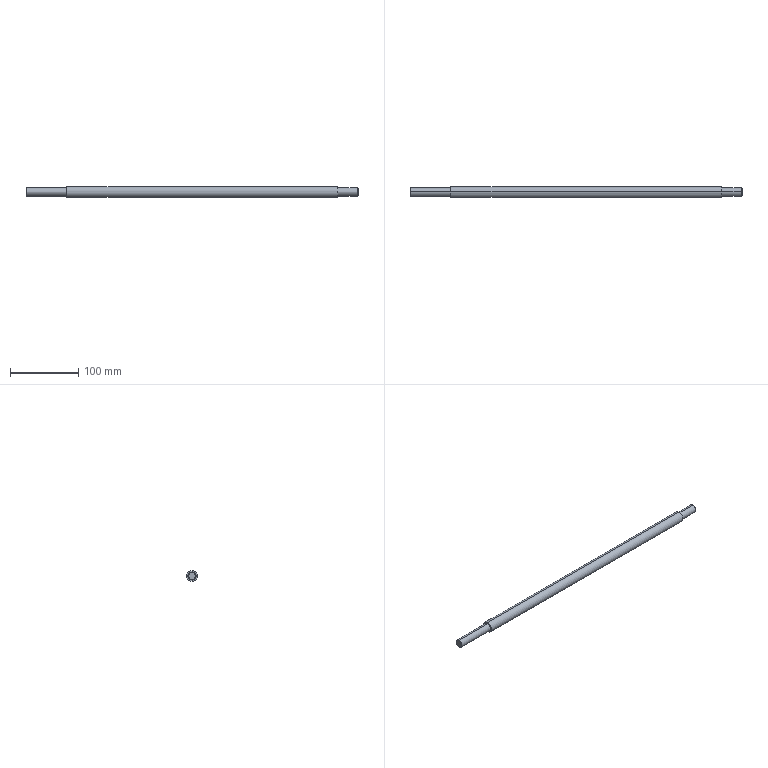Part | SolidWorks | features ICE 4, Chamfer 2, Extrusion 1, Helix 1, SweepCut 1 | 1 solid | 14 faces | box 487 x 16 x 16 mm | volume 89965 mm3 | cylinder 6 | cone 4 | plane 4 | commonest cylinder face diameters 12 x4 16 x2
STEP:
#1=CARTESIAN_POINT('',(-258.5,0.,5.));
#2=VERTEX_POINT('',#1);
#3=CARTESIAN_POINT('',(-258.5,0.,-5.));
#4=VERTEX_POINT('',#3);
#5=CARTESIAN_POINT('',(-258.5,0.,0.));
#6=DIRECTION('',(-1.,0.,0.));
#7=DIRECTION('',(0.,0.,1.));
#8=AXIS2_PLACEMENT_3D('',#5,#6,#7);
#9=CIRCLE('',#8,5.);
#10=EDGE_CURVE('',#2,#4,#9,.T.);
#11=ORIENTED_EDGE('',*,*,#10,.F.);
#12=CARTESIAN_POINT('',(-257.5,0.,6.));
#13=VERTEX_POINT('',#12);
#14=CARTESIAN_POINT('',(-258.5,0.,5.));
#15=DIRECTION('',(0.7071,0.,0.7071));
#16=VECTOR('',#15,1000.);
#17=LINE('',#14,#16);
#18=EDGE_CURVE('',#2,#13,#17,.T.);
#19=ORIENTED_EDGE('',*,*,#18,.T.);
#20=CARTESIAN_POINT('',(-257.5,0.,-6.));
#21=VERTEX_POINT('',#20);
#22=CARTESIAN_POINT('',(-257.5,0.,0.));
#23=DIRECTION('',(1.,0.,0.));
#24=DIRECTION('',(0.,0.,1.));
#25=AXIS2_PLACEMENT_3D('',#22,#23,#24);
#26=CIRCLE('',#25,6.);
#27=EDGE_CURVE('',#21,#13,#26,.T.);
#28=ORIENTED_EDGE('',*,*,#27,.F.);
#29=CARTESIAN_POINT('',(-258.5,0.,-5.));
#30=DIRECTION('',(0.7071,0.,-0.7071));
#31=VECTOR('',#30,1000.);
#32=LINE('',#29,#31);
#33=EDGE_CURVE('',#4,#21,#32,.T.);
#34=ORIENTED_EDGE('',*,*,#33,.F.);
#35=EDGE_LOOP('',(#11,#19,#28,#34));
#36=FACE_OUTER_BOUND('',#35,.T.);
#37=CARTESIAN_POINT('',(-258.5,0.,0.));
#38=DIRECTION('',(1.,0.,0.));
#39=DIRECTION('',(0.,0.,-1.));
#40=AXIS2_PLACEMENT_3D('',#37,#38,#39);
#41=CONICAL_SURFACE('',#40,5.,0.7854);
#42=ADVANCED_FACE('',(#36),#41,.T.);
#43=CARTESIAN_POINT('',(228.5,0.,-5.));
#44=VERTEX_POINT('',#43);
#45=CARTESIAN_POINT('',(228.5,0.,5.));
#46=VERTEX_POINT('',#45);
#47=CARTESIAN_POINT('',(228.5,0.,0.));
#48=DIRECTION('',(1.,0.,0.));
#49=DIRECTION('',(0.,0.,-1.));
#50=AXIS2_PLACEMENT_3D('',#47,#48,#49);
#51=CIRCLE('',#50,5.);
#52=EDGE_CURVE('',#44,#46,#51,.T.);
#53=ORIENTED_EDGE('',*,*,#52,.F.);
#54=CARTESIAN_POINT('',(227.5,0.,-6.));
#55=VERTEX_POINT('',#54);
#56=CARTESIAN_POINT('',(228.5,0.,-5.));
#57=DIRECTION('',(-0.7071,0.,-0.7071));
#58=VECTOR('',#57,1000.);
#59=LINE('',#56,#58);
#60=EDGE_CURVE('',#44,#55,#59,.T.);
#61=ORIENTED_EDGE('',*,*,#60,.T.);
#62=CARTESIAN_POINT('',(227.5,0.,6.));
#63=VERTEX_POINT('',#62);
#64=CARTESIAN_POINT('',(227.5,0.,0.));
#65=DIRECTION('',(-1.,0.,0.));
#66=DIRECTION('',(0.,0.,-1.));
#67=AXIS2_PLACEMENT_3D('',#64,#65,#66);
#68=CIRCLE('',#67,6.);
#69=EDGE_CURVE('',#63,#55,#68,.T.);
#70=ORIENTED_EDGE('',*,*,#69,.F.);
#71=CARTESIAN_POINT('',(228.5,0.,5.));
#72=DIRECTION('',(-0.7071,0.,0.7071));
#73=VECTOR('',#72,1000.);
#74=LINE('',#71,#73);
#75=EDGE_CURVE('',#46,#63,#74,.T.);
#76=ORIENTED_EDGE('',*,*,#75,.F.);
#77=EDGE_LOOP('',(#53,#61,#70,#76));
#78=FACE_OUTER_BOUND('',#77,.T.);
#79=CARTESIAN_POINT('',(228.5,0.,0.));
#80=DIRECTION('',(-1.,0.,0.));
#81=DIRECTION('',(0.,0.,1.));
#82=AXIS2_PLACEMENT_3D('',#79,#80,#81);
#83=CONICAL_SURFACE('',#82,5.,0.7854);
#84=ADVANCED_FACE('',(#78),#83,.T.);
#85=ORIENTED_EDGE('',*,*,#27,.T.);
#86=CARTESIAN_POINT('',(-198.5,0.,6.));
#87=VERTEX_POINT('',#86);
#88=CARTESIAN_POINT('',(-258.5,0.,6.));
#89=DIRECTION('',(1.,0.,0.));
#90=VECTOR('',#89,1000.);
#91=LINE('',#88,#90);
#92=EDGE_CURVE('',#13,#87,#91,.T.);
#93=ORIENTED_EDGE('',*,*,#92,.T.);
#94=CARTESIAN_POINT('',(-198.5,0.,-6.));
#95=VERTEX_POINT('',#94);
#96=CARTESIAN_POINT('',(-198.5,0.,0.));
#97=DIRECTION('',(-1.,0.,0.));
#98=DIRECTION('',(0.,0.,1.));
#99=AXIS2_PLACEMENT_3D('',#96,#97,#98);
#100=CIRCLE('',#99,6.);
#101=EDGE_CURVE('',#87,#95,#100,.T.);
#102=ORIENTED_EDGE('',*,*,#101,.T.);
#103=CARTESIAN_POINT('',(-258.5,0.,-6.));
#104=DIRECTION('',(1.,0.,0.));
#105=VECTOR('',#104,1000.);
#106=LINE('',#103,#105);
#107=EDGE_CURVE('',#21,#95,#106,.T.);
#108=ORIENTED_EDGE('',*,*,#107,.F.);
#109=EDGE_LOOP('',(#85,#93,#102,#108));
#110=FACE_OUTER_BOUND('',#109,.T.);
#111=CARTESIAN_POINT('',(-258.5,0.,0.));
#112=DIRECTION('',(1.,0.,0.));
#113=DIRECTION('',(0.,0.,-1.));
#114=AXIS2_PLACEMENT_3D('',#111,#112,#113);
#115=CYLINDRICAL_SURFACE('',#114,6.);
#116=ADVANCED_FACE('',(#110),#115,.T.);
#117=ORIENTED_EDGE('',*,*,#69,.T.);
#118=CARTESIAN_POINT('',(198.5,0.,-6.));
#119=VERTEX_POINT('',#118);
#120=CARTESIAN_POINT('',(228.5,0.,-6.));
#121=DIRECTION('',(-1.,0.,0.));
#122=VECTOR('',#121,1000.);
#123=LINE('',#120,#122);
#124=EDGE_CURVE('',#55,#119,#123,.T.);
#125=ORIENTED_EDGE('',*,*,#124,.T.);
#126=CARTESIAN_POINT('',(198.5,0.,6.));
#127=VERTEX_POINT('',#126);
#128=CARTESIAN_POINT('',(198.5,0.,0.));
#129=DIRECTION('',(1.,0.,0.));
#130=DIRECTION('',(0.,0.,-1.));
#131=AXIS2_PLACEMENT_3D('',#128,#129,#130);
#132=CIRCLE('',#131,6.);
#133=EDGE_CURVE('',#119,#127,#132,.T.);
#134=ORIENTED_EDGE('',*,*,#133,.T.);
#135=CARTESIAN_POINT('',(228.5,0.,6.));
#136=DIRECTION('',(-1.,0.,0.));
#137=VECTOR('',#136,1000.);
#138=LINE('',#135,#137);
#139=EDGE_CURVE('',#63,#127,#138,.T.);
#140=ORIENTED_EDGE('',*,*,#139,.F.);
#141=EDGE_LOOP('',(#117,#125,#134,#140));
#142=FACE_OUTER_BOUND('',#141,.T.);
#143=CARTESIAN_POINT('',(228.5,0.,0.));
#144=DIRECTION('',(-1.,0.,0.));
#145=DIRECTION('',(0.,0.,1.));
#146=AXIS2_PLACEMENT_3D('',#143,#144,#145);
#147=CYLINDRICAL_SURFACE('',#146,6.);
#148=ADVANCED_FACE('',(#142),#147,.T.);
#149=CARTESIAN_POINT('',(198.5,0.,-8.));
#150=VERTEX_POINT('',#149);
#151=CARTESIAN_POINT('',(198.5,0.,8.));
#152=VERTEX_POINT('',#151);
#153=CARTESIAN_POINT('',(198.5,0.,0.));
#154=DIRECTION('',(1.,0.,0.));
#155=DIRECTION('',(0.,0.,-1.));
#156=AXIS2_PLACEMENT_3D('',#153,#154,#155);
#157=CIRCLE('',#156,8.);
#158=EDGE_CURVE('',#150,#152,#157,.T.);
#159=ORIENTED_EDGE('',*,*,#158,.F.);
#160=CARTESIAN_POINT('',(-198.5,0.,-8.));
#161=VERTEX_POINT('',#160);
#162=CARTESIAN_POINT('',(198.5,0.,-8.));
#163=DIRECTION('',(-1.,0.,0.));
#164=VECTOR('',#163,1000.);
#165=LINE('',#162,#164);
#166=EDGE_CURVE('',#150,#161,#165,.T.);
#167=ORIENTED_EDGE('',*,*,#166,.T.);
#168=CARTESIAN_POINT('',(-198.5,0.,8.));
#169=VERTEX_POINT('',#168);
#170=CARTESIAN_POINT('',(-198.5,0.,0.));
#171=DIRECTION('',(1.,0.,0.));
#172=DIRECTION('',(0.,0.,-1.));
#173=AXIS2_PLACEMENT_3D('',#170,#171,#172);
#174=CIRCLE('',#173,8.);
#175=EDGE_CURVE('',#161,#169,#174,.T.);
#176=ORIENTED_EDGE('',*,*,#175,.T.);
#177=CARTESIAN_POINT('',(198.5,0.,8.));
#178=DIRECTION('',(-1.,0.,0.));
#179=VECTOR('',#178,1000.);
#180=LINE('',#177,#179);
#181=EDGE_CURVE('',#152,#169,#180,.T.);
#182=ORIENTED_EDGE('',*,*,#181,.F.);
#183=EDGE_LOOP('',(#159,#167,#176,#182));
#184=FACE_OUTER_BOUND('',#183,.T.);
#185=CARTESIAN_POINT('',(198.5,0.,0.));
#186=DIRECTION('',(-1.,0.,0.));
#187=DIRECTION('',(0.,0.,1.));
#188=AXIS2_PLACEMENT_3D('',#185,#186,#187);
#189=CYLINDRICAL_SURFACE('',#188,8.);
#190=ADVANCED_FACE('',(#184),#189,.T.);
#191=ORIENTED_EDGE('',*,*,#166,.F.);
#192=CARTESIAN_POINT('',(198.5,0.,0.));
#193=DIRECTION('',(1.,0.,0.));
#194=DIRECTION('',(0.,0.,-1.));
#195=AXIS2_PLACEMENT_3D('',#192,#193,#194);
#196=CIRCLE('',#195,8.);
#197=EDGE_CURVE('',#152,#150,#196,.T.);
#198=ORIENTED_EDGE('',*,*,#197,.F.);
#199=ORIENTED_EDGE('',*,*,#181,.T.);
#200=CARTESIAN_POINT('',(-198.5,0.,0.));
#201=DIRECTION('',(1.,0.,0.));
#202=DIRECTION('',(0.,0.,-1.));
#203=AXIS2_PLACEMENT_3D('',#200,#201,#202);
#204=CIRCLE('',#203,8.);
#205=EDGE_CURVE('',#169,#161,#204,.T.);
#206=ORIENTED_EDGE('',*,*,#205,.T.);
#207=EDGE_LOOP('',(#191,#198,#199,#206));
#208=FACE_OUTER_BOUND('',#207,.T.);
#209=CARTESIAN_POINT('',(198.5,0.,0.));
#210=DIRECTION('',(-1.,0.,0.));
#211=DIRECTION('',(0.,0.,1.));
#212=AXIS2_PLACEMENT_3D('',#209,#210,#211);
#213=CYLINDRICAL_SURFACE('',#212,8.);
#214=ADVANCED_FACE('',(#208),#213,.T.);
#215=CARTESIAN_POINT('',(198.5,0.,0.));
#216=DIRECTION('',(1.,0.,0.));
#217=DIRECTION('',(0.,0.,-1.));
#218=AXIS2_PLACEMENT_3D('',#215,#216,#217);
#219=CIRCLE('',#218,6.);
#220=EDGE_CURVE('',#127,#119,#219,.T.);
#221=ORIENTED_EDGE('',*,*,#220,.F.);
#222=ORIENTED_EDGE('',*,*,#133,.F.);
#223=EDGE_LOOP('',(#221,#222));
#224=FACE_BOUND('',#223,.T.);
#225=ORIENTED_EDGE('',*,*,#197,.T.);
#226=ORIENTED_EDGE('',*,*,#158,.T.);
#227=EDGE_LOOP('',(#225,#226));
#228=FACE_OUTER_BOUND('',#227,.T.);
#229=CARTESIAN_POINT('',(198.5,0.,0.));
#230=DIRECTION('',(1.,0.,0.));
#231=DIRECTION('',(0.,0.,-1.));
#232=AXIS2_PLACEMENT_3D('',#229,#230,#231);
#233=PLANE('',#232);
#234=ADVANCED_FACE('',(#224,#228),#233,.T.);
#235=CARTESIAN_POINT('',(-198.5,0.,0.));
#236=DIRECTION('',(-1.,0.,0.));
#237=DIRECTION('',(0.,0.,1.));
#238=AXIS2_PLACEMENT_3D('',#235,#236,#237);
#239=CIRCLE('',#238,6.);
#240=EDGE_CURVE('',#95,#87,#239,.T.);
#241=ORIENTED_EDGE('',*,*,#240,.F.);
#242=ORIENTED_EDGE('',*,*,#101,.F.);
#243=EDGE_LOOP('',(#241,#242));
#244=FACE_BOUND('',#243,.T.);
#245=ORIENTED_EDGE('',*,*,#205,.F.);
#246=ORIENTED_EDGE('',*,*,#175,.F.);
#247=EDGE_LOOP('',(#245,#246));
#248=FACE_OUTER_BOUND('',#247,.T.);
#249=CARTESIAN_POINT('',(-198.5,0.,0.));
#250=DIRECTION('',(1.,0.,0.));
#251=DIRECTION('',(0.,0.,-1.));
#252=AXIS2_PLACEMENT_3D('',#249,#250,#251);
#253=PLANE('',#252);
#254=ADVANCED_FACE('',(#244,#248),#253,.F.);
#255=ORIENTED_EDGE('',*,*,#124,.F.);
#256=CARTESIAN_POINT('',(227.5,0.,0.));
#257=DIRECTION('',(-1.,0.,0.));
#258=DIRECTION('',(0.,0.,-1.));
#259=AXIS2_PLACEMENT_3D('',#256,#257,#258);
#260=CIRCLE('',#259,6.);
#261=EDGE_CURVE('',#55,#63,#260,.T.);
#262=ORIENTED_EDGE('',*,*,#261,.T.);
#263=ORIENTED_EDGE('',*,*,#139,.T.);
#264=ORIENTED_EDGE('',*,*,#220,.T.);
#265=EDGE_LOOP('',(#255,#262,#263,#264));
#266=FACE_OUTER_BOUND('',#265,.T.);
#267=CARTESIAN_POINT('',(228.5,0.,0.));
#268=DIRECTION('',(-1.,0.,0.));
#269=DIRECTION('',(0.,0.,1.));
#270=AXIS2_PLACEMENT_3D('',#267,#268,#269);
#271=CYLINDRICAL_SURFACE('',#270,6.);
#272=ADVANCED_FACE('',(#266),#271,.T.);
#273=CARTESIAN_POINT('',(228.5,0.,0.));
#274=DIRECTION('',(1.,0.,0.));
#275=DIRECTION('',(0.,0.,-1.));
#276=AXIS2_PLACEMENT_3D('',#273,#274,#275);
#277=CIRCLE('',#276,5.);
#278=EDGE_CURVE('',#46,#44,#277,.T.);
#279=ORIENTED_EDGE('',*,*,#278,.T.);
#280=ORIENTED_EDGE('',*,*,#52,.T.);
#281=EDGE_LOOP('',(#279,#280));
#282=FACE_OUTER_BOUND('',#281,.T.);
#283=CARTESIAN_POINT('',(228.5,0.,0.));
#284=DIRECTION('',(1.,0.,0.));
#285=DIRECTION('',(0.,0.,-1.));
#286=AXIS2_PLACEMENT_3D('',#283,#284,#285);
#287=PLANE('',#286);
#288=ADVANCED_FACE('',(#282),#287,.T.);
#289=ORIENTED_EDGE('',*,*,#92,.F.);
#290=CARTESIAN_POINT('',(-257.5,0.,0.));
#291=DIRECTION('',(1.,0.,0.));
#292=DIRECTION('',(0.,0.,1.));
#293=AXIS2_PLACEMENT_3D('',#290,#291,#292);
#294=CIRCLE('',#293,6.);
#295=EDGE_CURVE('',#13,#21,#294,.T.);
#296=ORIENTED_EDGE('',*,*,#295,.T.);
#297=ORIENTED_EDGE('',*,*,#107,.T.);
#298=ORIENTED_EDGE('',*,*,#240,.T.);
#299=EDGE_LOOP('',(#289,#296,#297,#298));
#300=FACE_OUTER_BOUND('',#299,.T.);
#301=CARTESIAN_POINT('',(-258.5,0.,0.));
#302=DIRECTION('',(1.,0.,0.));
#303=DIRECTION('',(0.,0.,-1.));
#304=AXIS2_PLACEMENT_3D('',#301,#302,#303);
#305=CYLINDRICAL_SURFACE('',#304,6.);
#306=ADVANCED_FACE('',(#300),#305,.T.);
#307=CARTESIAN_POINT('',(-258.5,0.,0.));
#308=DIRECTION('',(-1.,0.,0.));
#309=DIRECTION('',(0.,0.,1.));
#310=AXIS2_PLACEMENT_3D('',#307,#308,#309);
#311=CIRCLE('',#310,5.);
#312=EDGE_CURVE('',#4,#2,#311,.T.);
#313=ORIENTED_EDGE('',*,*,#312,.T.);
#314=ORIENTED_EDGE('',*,*,#10,.T.);
#315=EDGE_LOOP('',(#313,#314));
#316=FACE_OUTER_BOUND('',#315,.T.);
#317=CARTESIAN_POINT('',(-258.5,0.,0.));
#318=DIRECTION('',(-1.,0.,0.));
#319=DIRECTION('',(0.,0.,1.));
#320=AXIS2_PLACEMENT_3D('',#317,#318,#319);
#321=PLANE('',#320);
#322=ADVANCED_FACE('',(#316),#321,.T.);
#323=ORIENTED_EDGE('',*,*,#60,.F.);
#324=ORIENTED_EDGE('',*,*,#278,.F.);
#325=ORIENTED_EDGE('',*,*,#75,.T.);
#326=ORIENTED_EDGE('',*,*,#261,.F.);
#327=EDGE_LOOP('',(#323,#324,#325,#326));
#328=FACE_OUTER_BOUND('',#327,.T.);
#329=CARTESIAN_POINT('',(228.5,0.,0.));
#330=DIRECTION('',(-1.,0.,0.));
#331=DIRECTION('',(0.,0.,1.));
#332=AXIS2_PLACEMENT_3D('',#329,#330,#331);
#333=CONICAL_SURFACE('',#332,5.,0.7854);
#334=ADVANCED_FACE('',(#328),#333,.T.);
#335=ORIENTED_EDGE('',*,*,#18,.F.);
#336=ORIENTED_EDGE('',*,*,#312,.F.);
#337=ORIENTED_EDGE('',*,*,#33,.T.);
#338=ORIENTED_EDGE('',*,*,#295,.F.);
#339=EDGE_LOOP('',(#335,#336,#337,#338));
#340=FACE_OUTER_BOUND('',#339,.T.);
#341=CARTESIAN_POINT('',(-258.5,0.,0.));
#342=DIRECTION('',(1.,0.,0.));
#343=DIRECTION('',(0.,0.,-1.));
#344=AXIS2_PLACEMENT_3D('',#341,#342,#343);
#345=CONICAL_SURFACE('',#344,5.,0.7854);
#346=ADVANCED_FACE('',(#340),#345,.T.);
#347=CLOSED_SHELL('',(#42,#84,#116,#148,#190,#214,#234,#254,#272,#288,#306,#322,#334,#346));
#348=MANIFOLD_SOLID_BREP('',#347);
#349=CARTESIAN_POINT('',(0.,0.,0.));
#350=DIRECTION('',(0.,0.,1.));
#351=DIRECTION('',(1.,0.,0.));
#352=AXIS2_PLACEMENT_3D('',#349,#350,#351);
#353=(LENGTH_UNIT()NAMED_UNIT(*)SI_UNIT(.MILLI.,.METRE.));
#354=UNCERTAINTY_MEASURE_WITH_UNIT(LENGTH_MEASURE(0.00001),#353,'','');
#355=(NAMED_UNIT(*)PLANE_ANGLE_UNIT()SI_UNIT($,.RADIAN.));
#356=(NAMED_UNIT(*)SI_UNIT($,.STERADIAN.)SOLID_ANGLE_UNIT());
#357=(GEOMETRIC_REPRESENTATION_CONTEXT(3)GLOBAL_UNCERTAINTY_ASSIGNED_CONTEXT((#354))GLOBAL_UNIT_ASSIGNED_CONTEXT((#353,#355,#356))REPRESENTATION_CONTEXT('',''));
#358=ADVANCED_BREP_SHAPE_REPRESENTATION('',(#348,#352),#357);